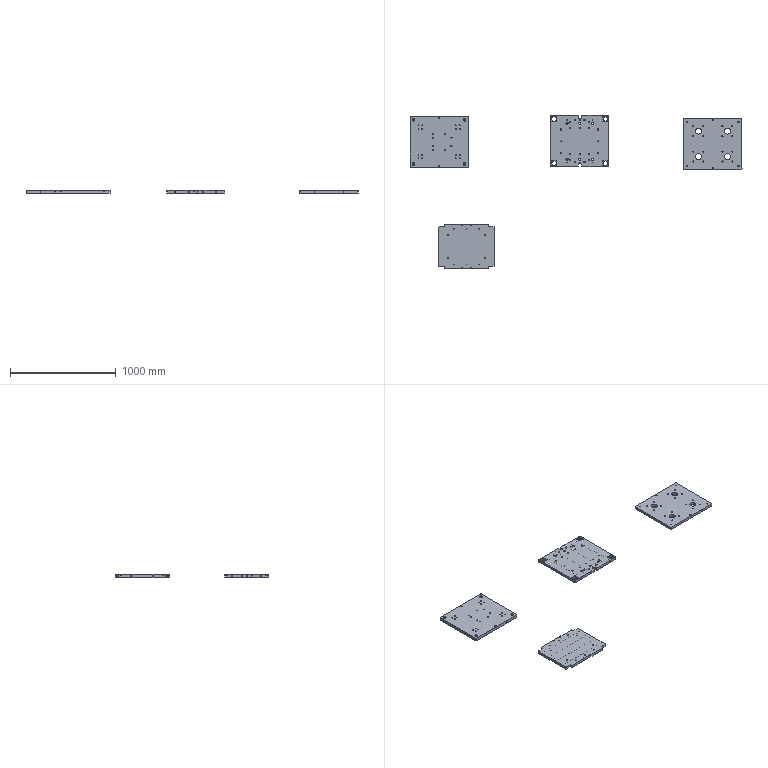NC program | Mastercam | posted with a generic post | part box 3140 x 1452 x 30 mm
Lines 481 to 2018 of 5015:
N4780 T16 M6
N4790 G0 G90 G17 G54 X-276. Y206. A0. S6000 M3
N4800 G43 H16 Z50. M8
N4810 Z1.
N4820 G1 Z-.499 F600.
N4830 X-260. F4000.
N4840 X-226.
N4850 Y212.5
N4860 Y228.5
N4870 Z-.998 F600.
N4880 Y212.5 F4000.
N4890 Y206.
N4900 X-260.
N4910 X-276.
N4920 Z-1.497 F600.
N4930 X-260. F4000.
N4940 X-226.
N4950 Y212.5
N4960 Y228.5
N4970 Z-1.996 F600.
N4980 Y212.5 F4000.
N4990 Y206.
N5000 X-260.
N5010 X-276.
N5020 Z-2.495 F600.
N5030 X-260. F4000.
N5040 X-226.
N5050 Y212.5
N5060 Y228.5
N5070 Z-2.994 F600.
N5080 Y212.5 F4000.
N5090 Y206.
N5100 X-260.
N5110 X-276.
N5120 Z-3.493 F600.
N5130 X-260. F4000.
N5140 X-226.
N5150 Y212.5
N5160 Y228.5
N5170 Z-3.992 F600.
N5180 Y212.5 F4000.
N5190 Y206.
N5200 X-260.
N5210 X-276.
N5220 Z-4.491 F600.
N5230 X-260. F4000.
N5240 X-226.
N5250 Y212.5
N5260 Y228.5
N5270 Z-4.99 F600.
N5280 Y212.5 F4000.
N5290 Y206.
N5300 X-260.
N5310 X-276.
N5320 Z-5.489 F600.
N5330 X-260. F4000.
N5340 X-226.
N5350 Y212.5
N5360 Y228.5
N5370 Z-5.988 F600.
N5380 Y212.5 F4000.
N5390 Y206.
N5400 X-260.
N5410 X-276.
N5420 Z-6.487 F600.
N5430 X-260. F4000.
N5440 X-226.
N5450 Y212.5
N5460 Y228.5
N5470 Z-6.986 F600.
N5480 Y212.5 F4000.
N5490 Y206.
N5500 X-260.
N5510 X-276.
N5520 Z-7.485 F600.
N5530 X-260. F4000.
N5540 X-226.
N5550 Y212.5
N5560 Y228.5
N5570 Z-7.984 F600.
N5580 Y212.5 F4000.
N5590 Y206.
N5600 X-260.
N5610 X-276.
N5620 Z-8.483 F600.
N5630 X-260. F4000.
N5640 X-226.
N5650 Y212.5
N5660 Y228.5
N5670 Z-8.982 F600.
N5680 Y212.5 F4000.
N5690 Y206.
N5700 X-260.
N5710 X-276.
N5720 Z-9.481 F600.
N5730 X-260. F4000.
N5740 X-226.
N5750 Y212.5
N5760 Y228.5
N5770 Z-9.98 F600.
N5780 Y212.5 F4000.
N5790 Y206.
N5800 X-260.
N5810 X-276.
N5820 Z-10.479 F600.
N5830 X-260. F4000.
N5840 X-226.
N5850 Y212.5
N5860 Y228.5
N5870 Z-10.978 F600.
N5880 Y212.5 F4000.
N5890 Y206.
N5900 X-260.
N5910 X-276.
N5920 Z-11.477 F600.
N5930 X-260. F4000.
N5940 X-226.
N5950 Y212.5
N5960 Y228.5
N5970 Z-11.976 F600.
N5980 Y212.5 F4000.
N5990 Y206.
N6000 X-260.
N6010 X-276.
N6020 Z-12.475 F600.
N6030 X-260. F4000.
N6040 X-226.
N6050 Y212.5
N6060 Y228.5
N6070 Z-12.974 F600.
N6080 Y212.5 F4000.
N6090 Y206.
N6100 X-260.
N6110 X-276.
N6120 Z-13.473 F600.
N6130 X-260. F4000.
N6140 X-226.
N6150 Y212.5
N6160 Y228.5
N6170 Z-13.972 F600.
N6180 Y212.5 F4000.
N6190 Y206.
N6200 X-260.
N6210 X-276.
N6220 Z-14.471 F600.
N6230 X-260. F4000.
N6240 X-226.
N6250 Y212.5
N6260 Y228.5
N6270 Z-14.97 F600.
N6280 Y212.5 F4000.
N6290 Y206.
N6300 X-260.
N6310 X-276.
N6320 Z-15.469 F600.
N6330 X-260. F4000.
N6340 X-226.
N6350 Y212.5
N6360 Y228.5
N6370 Z-15.968 F600.
N6380 Y212.5 F4000.
N6390 Y206.
N6400 X-260.
N6410 X-276.
N6420 Z-16.467 F600.
N6430 X-260. F4000.
N6440 X-226.
N6450 Y212.5
N6460 Y228.5
N6470 Z-16.966 F600.
N6480 Y212.5 F4000.
N6490 Y206.
N6500 X-260.
N6510 X-276.
N6520 Z-17.465 F600.
N6530 X-260. F4000.
N6540 X-226.
N6550 Y212.5
N6560 Y228.5
N6570 Z-17.964 F600.
N6580 Y212.5 F4000.
N6590 Y206.
N6600 X-260.
N6610 X-276.
N6620 Z-18.463 F600.
N6630 X-260. F4000.
N6640 X-226.
N6650 Y212.5
N6660 Y228.5
N6670 Z-18.962 F600.
N6680 Y212.5 F4000.
N6690 Y206.
N6700 X-260.
N6710 X-276.
N6720 Z-19.461 F600.
N6730 X-260. F4000.
N6740 X-226.
N6750 Y212.5
N6760 Y228.5
N6770 Z-19.96 F600.
N6780 Y212.5 F4000.
N6790 Y206.
N6800 X-260.
N6810 X-276.
N6820 Z-20.459 F600.
N6830 X-260. F4000.
N6840 X-226.
N6850 Y212.5
N6860 Y228.5
N6870 Z-20.958 F600.
N6880 Y212.5 F4000.
N6890 Y206.
N6900 X-260.
N6910 X-276.
N6920 Z-21.457 F600.
N6930 X-260. F4000.
N6940 X-226.
N6950 Y212.5
N6960 Y228.5
N6970 Z-21.956 F600.
N6980 Y212.5 F4000.
N6990 Y206.
N7000 X-260.
N7010 X-276.
N7020 Z-22.455 F600.
N7030 X-260. F4000.
N7040 X-226.
N7050 Y212.5
N7060 Y228.5
N7070 Z-22.954 F600.
N7080 Y212.5 F4000.
N7090 Y206.
N7100 X-260.
N7110 X-276.
N7120 Z-23.453 F600.
N7130 X-260. F4000.
N7140 X-226.
N7150 Y212.5
N7160 Y228.5
N7170 Z-23.952 F600.
N7180 Y212.5 F4000.
N7190 Y206.
N7200 X-260.
N7210 X-276.
N7220 Z-24.451 F600.
N7230 X-260. F4000.
N7240 X-226.
N7250 Y212.5
N7260 Y228.5
N7270 Z-24.95 F600.
N7280 Y212.5 F4000.
N7290 Y206.
N7300 X-260.
N7310 X-276.
N7320 G0 Z50.
N7330 Y198.
N7340 Z1.
N7350 G1 Z-.499 F600.
N7360 X-260. F4000.
N7370 X-218.
N7380 Y212.5
N7390 Y228.5
N7400 Z-.998 F600.
N7410 Y212.5 F4000.
N7420 Y198.
N7430 X-260.
N7440 X-276.
N7450 Z-1.497 F600.
N7460 X-260. F4000.
N7470 X-218.
N7480 Y212.5
N7490 Y228.5
N7500 Z-1.996 F600.
N7510 Y212.5 F4000.
N7520 Y198.
N7530 X-260.
N7540 X-276.
N7550 Z-2.495 F600.
N7560 X-260. F4000.
N7570 X-218.
N7580 Y212.5
N7590 Y228.5
N7600 Z-2.994 F600.
N7610 Y212.5 F4000.
N7620 Y198.
N7630 X-260.
N7640 X-276.
N7650 Z-3.493 F600.
N7660 X-260. F4000.
N7670 X-218.
N7680 Y212.5
N7690 Y228.5
N7700 Z-3.992 F600.
N7710 Y212.5 F4000.
N7720 Y198.
N7730 X-260.
N7740 X-276.
N7750 Z-4.491 F600.
N7760 X-260. F4000.
N7770 X-218.
N7780 Y212.5
N7790 Y228.5
N7800 Z-4.99 F600.
N7810 Y212.5 F4000.
N7820 Y198.
N7830 X-260.
N7840 X-276.
N7850 Z-5.489 F600.
N7860 X-260. F4000.
N7870 X-218.
N7880 Y212.5
N7890 Y228.5
N7900 Z-5.988 F600.
N7910 Y212.5 F4000.
N7920 Y198.
N7930 X-260.
N7940 X-276.
N7950 Z-6.487 F600.
N7960 X-260. F4000.
N7970 X-218.
N7980 Y212.5
N7990 Y228.5
N8000 Z-6.986 F600.
N8010 Y212.5 F4000.
N8020 Y198.
N8030 X-260.
N8040 X-276.
N8050 Z-7.485 F600.
N8060 X-260. F4000.
N8070 X-218.
N8080 Y212.5
N8090 Y228.5
N8100 Z-7.984 F600.
N8110 Y212.5 F4000.
N8120 Y198.
N8130 X-260.
N8140 X-276.
N8150 Z-8.483 F600.
N8160 X-260. F4000.
N8170 X-218.
N8180 Y212.5
N8190 Y228.5
N8200 Z-8.982 F600.
N8210 Y212.5 F4000.
N8220 Y198.
N8230 X-260.
N8240 X-276.
N8250 Z-9.481 F600.
N8260 X-260. F4000.
N8270 X-218.
N8280 Y212.5
N8290 Y228.5
N8300 Z-9.98 F600.
N8310 Y212.5 F4000.
N8320 Y198.
N8330 X-260.
N8340 X-276.
N8350 Z-10.479 F600.
N8360 X-260. F4000.
N8370 X-218.
N8380 Y212.5
N8390 Y228.5
N8400 Z-10.978 F600.
N8410 Y212.5 F4000.
N8420 Y198.
N8430 X-260.
N8440 X-276.
N8450 Z-11.477 F600.
N8460 X-260. F4000.
N8470 X-218.
N8480 Y212.5
N8490 Y228.5
N8500 Z-11.976 F600.
N8510 Y212.5 F4000.
N8520 Y198.
N8530 X-260.
N8540 X-276.
N8550 Z-12.475 F600.
N8560 X-260. F4000.
N8570 X-218.
N8580 Y212.5
N8590 Y228.5
N8600 Z-12.974 F600.
N8610 Y212.5 F4000.
N8620 Y198.
N8630 X-260.
N8640 X-276.
N8650 Z-13.473 F600.
N8660 X-260. F4000.
N8670 X-218.
N8680 Y212.5
N8690 Y228.5
N8700 Z-13.972 F600.
N8710 Y212.5 F4000.
N8720 Y198.
N8730 X-260.
N8740 X-276.
N8750 Z-14.471 F600.
N8760 X-260. F4000.
N8770 X-218.
N8780 Y212.5
N8790 Y228.5
N8800 Z-14.97 F600.
N8810 Y212.5 F4000.
N8820 Y198.
N8830 X-260.
N8840 X-276.
N8850 Z-15.469 F600.
N8860 X-260. F4000.
N8870 X-218.
N8880 Y212.5
N8890 Y228.5
N8900 Z-15.968 F600.
N8910 Y212.5 F4000.
N8920 Y198.
N8930 X-260.
N8940 X-276.
N8950 Z-16.467 F600.
N8960 X-260. F4000.
N8970 X-218.
N8980 Y212.5
N8990 Y228.5
N9000 Z-16.966 F600.
N9010 Y212.5 F4000.
N9020 Y198.
N9030 X-260.
N9040 X-276.
N9050 Z-17.465 F600.
N9060 X-260. F4000.
N9070 X-218.
N9080 Y212.5
N9090 Y228.5
N9100 Z-17.964 F600.
N9110 Y212.5 F4000.
N9120 Y198.
N9130 X-260.
N9140 X-276.
N9150 Z-18.463 F600.
N9160 X-260. F4000.
N9170 X-218.
N9180 Y212.5
N9190 Y228.5
N9200 Z-18.962 F600.
N9210 Y212.5 F4000.
N9220 Y198.
N9230 X-260.
N9240 X-276.
N9250 Z-19.461 F600.
N9260 X-260. F4000.
N9270 X-218.
N9280 Y212.5
N9290 Y228.5
N9300 Z-19.96 F600.
N9310 Y212.5 F4000.
N9320 Y198.
N9330 X-260.
N9340 X-276.
N9350 Z-20.459 F600.
N9360 X-260. F4000.
N9370 X-218.
N9380 Y212.5
N9390 Y228.5
N9400 Z-20.958 F600.
N9410 Y212.5 F4000.
N9420 Y198.
N9430 X-260.
N9440 X-276.
N9450 Z-21.457 F600.
N9460 X-260. F4000.
N9470 X-218.
N9480 Y212.5
N9490 Y228.5
N9500 Z-21.956 F600.
N9510 Y212.5 F4000.
N9520 Y198.
N9530 X-260.
N9540 X-276.
N9550 Z-22.455 F600.
N9560 X-260. F4000.
N9570 X-218.
N9580 Y212.5
N9590 Y228.5
N9600 Z-22.954 F600.
N9610 Y212.5 F4000.
N9620 Y198.
N9630 X-260.
N9640 X-276.
N9650 Z-23.453 F600.
N9660 X-260. F4000.
N9670 X-218.
N9680 Y212.5
N9690 Y228.5
N9700 Z-23.952 F600.
N9710 Y212.5 F4000.
N9720 Y198.
N9730 X-260.
N9740 X-276.
N9750 Z-24.451 F600.
N9760 X-260. F4000.
N9770 X-218.
N9780 Y212.5
N9790 Y228.5
N9800 Z-24.95 F600.
N9810 Y212.5 F4000.
N9820 Y198.
N9830 X-260.
N9840 X-276.
N9850 G0 Z50.
N9860 X226. Y228.5
N9870 Z1.
N9880 G1 Z-.499 F600.
N9890 Y212.5 F4000.
N9900 Y206.
N9910 X260.
N9920 X276.
N9930 Z-.998 F600.
N9940 X260. F4000.
N9950 X226.
N9960 Y212.5
N9970 Y228.5
N9980 Z-1.497 F600.
N9990 Y212.5 F4000.
N100 Y206.
N110 X260.
N120 X276.
N130 Z-1.996 F600.
N140 X260. F4000.
N150 X226.
N160 Y212.5
N170 Y228.5
N180 Z-2.495 F600.
N190 Y212.5 F4000.
N200 Y206.
N210 X260.
N220 X276.
N230 Z-2.994 F600.
N240 X260. F4000.
N250 X226.
N260 Y212.5
N270 Y228.5
N280 Z-3.493 F600.
N290 Y212.5 F4000.
N300 Y206.
N310 X260.
N320 X276.
N330 Z-3.992 F600.
N340 X260. F4000.
N350 X226.
N360 Y212.5
N370 Y228.5
N380 Z-4.491 F600.
N390 Y212.5 F4000.
N400 Y206.
N410 X260.
N420 X276.
N430 Z-4.99 F600.
N440 X260. F4000.
N450 X226.
N460 Y212.5
N470 Y228.5
N480 Z-5.489 F600.
N490 Y212.5 F4000.
N500 Y206.
N510 X260.
N520 X276.
N530 Z-5.988 F600.
N540 X260. F4000.
N550 X226.
N560 Y212.5
N570 Y228.5
N580 Z-6.487 F600.
N590 Y212.5 F4000.
N600 Y206.
N610 X260.
N620 X276.
N630 Z-6.986 F600.
N640 X260. F4000.
N650 X226.
N660 Y212.5
N670 Y228.5
N680 Z-7.485 F600.
N690 Y212.5 F4000.
N700 Y206.
N710 X260.
N720 X276.
N730 Z-7.984 F600.
N740 X260. F4000.
N750 X226.
N760 Y212.5
N770 Y228.5
N780 Z-8.483 F600.
N790 Y212.5 F4000.
N800 Y206.
N810 X260.
N820 X276.
N830 Z-8.982 F600.
N840 X260. F4000.
N850 X226.
N860 Y212.5
N870 Y228.5
N880 Z-9.481 F600.
N890 Y212.5 F4000.
N900 Y206.
N910 X260.
N920 X276.
N930 Z-9.98 F600.
N940 X260. F4000.
N950 X226.
N960 Y212.5
N970 Y228.5
N980 Z-10.479 F600.
N990 Y212.5 F4000.
N1000 Y206.
N1010 X260.
N1020 X276.
N1030 Z-10.978 F600.
N1040 X260. F4000.
N1050 X226.
N1060 Y212.5
N1070 Y228.5
N1080 Z-11.477 F600.
N1090 Y212.5 F4000.
N1100 Y206.
N1110 X260.
N1120 X276.
N1130 Z-11.976 F600.
N1140 X260. F4000.
N1150 X226.
N1160 Y212.5
N1170 Y228.5
N1180 Z-12.475 F600.
N1190 Y212.5 F4000.
N1200 Y206.
N1210 X260.
N1220 X276.
N1230 Z-12.974 F600.
N1240 X260. F4000.
N1250 X226.
N1260 Y212.5
N1270 Y228.5
N1280 Z-13.473 F600.
N1290 Y212.5 F4000.
N1300 Y206.
N1310 X260.
N1320 X276.
N1330 Z-13.972 F600.
N1340 X260. F4000.
N1350 X226.
N1360 Y212.5
N1370 Y228.5
N1380 Z-14.471 F600.
N1390 Y212.5 F4000.
N1400 Y206.
N1410 X260.
N1420 X276.
N1430 Z-14.97 F600.
N1440 X260. F4000.
N1450 X226.
N1460 Y212.5
N1470 Y228.5
N1480 Z-15.469 F600.
N1490 Y212.5 F4000.
N1500 Y206.
N1510 X260.
N1520 X276.
N1530 Z-15.968 F600.
N1540 X260. F4000.
N1550 X226.
N1560 Y212.5
N1570 Y228.5
N1580 Z-16.467 F600.
N1590 Y212.5 F4000.
N1600 Y206.
N1610 X260.
N1620 X276.
N1630 Z-16.966 F600.
N1640 X260. F4000.
N1650 X226.
N1660 Y212.5
N1670 Y228.5
N1680 Z-17.465 F600.
N1690 Y212.5 F4000.
N1700 Y206.
N1710 X260.
N1720 X276.
N1730 Z-17.964 F600.
N1740 X260. F4000.
N1750 X226.
N1760 Y212.5
N1770 Y228.5
N1780 Z-18.463 F600.
N1790 Y212.5 F4000.
N1800 Y206.
N1810 X260.
N1820 X276.
N1830 Z-18.962 F600.
N1840 X260. F4000.
N1850 X226.
N1860 Y212.5
N1870 Y228.5
N1880 Z-19.461 F600.
N1890 Y212.5 F4000.
N1900 Y206.
N1910 X260.
N1920 X276.
N1930 Z-19.96 F600.
N1940 X260. F4000.
N1950 X226.
N1960 Y212.5
N1970 Y228.5
N1980 Z-20.459 F600.
N1990 Y212.5 F4000.
N2000 Y206.
N2010 X260.
N2020 X276.
N2030 Z-20.958 F600.
N2040 X260. F4000.
N2050 X226.
N2060 Y212.5
N2070 Y228.5
N2080 Z-21.457 F600.
N2090 Y212.5 F4000.
N2100 Y206.
N2110 X260.
N2120 X276.
N2130 Z-21.956 F600.
N2140 X260. F4000.
N2150 X226.
N2160 Y212.5
N2170 Y228.5
N2180 Z-22.455 F600.
N2190 Y212.5 F4000.
N2200 Y206.
N2210 X260.
N2220 X276.
N2230 Z-22.954 F600.
N2240 X260. F4000.
N2250 X226.
N2260 Y212.5
N2270 Y228.5
N2280 Z-23.453 F600.
N2290 Y212.5 F4000.
N2300 Y206.
N2310 X260.
N2320 X276.
N2330 Z-23.952 F600.
N2340 X260. F4000.
N2350 X226.
N2360 Y212.5
N2370 Y228.5
N2380 Z-24.451 F600.
N2390 Y212.5 F4000.
N2400 Y206.
N2410 X260.
N2420 X276.
N2430 Z-24.95 F600.
N2440 X260. F4000.
N2450 X226.
N2460 Y212.5
N2470 Y228.5
N2480 G0 Z50.
N2490 X218.
N2500 Z1.
N2510 G1 Z-.499 F600.
N2520 Y212.5 F4000.
N2530 Y198.
N2540 X260.
N2550 X276.
N2560 Z-.998 F600.
N2570 X260. F4000.
N2580 X218.
N2590 Y212.5
N2600 Y228.5
N2610 Z-1.497 F600.
N2620 Y212.5 F4000.
N2630 Y198.
N2640 X260.
N2650 X276.
N2660 Z-1.996 F600.
N2670 X260. F4000.
N2680 X218.
N2690 Y212.5
N2700 Y228.5
N2710 Z-2.495 F600.
N2720 Y212.5 F4000.
N2730 Y198.
N2740 X260.
N2750 X276.
N2760 Z-2.994 F600.
N2770 X260. F4000.
N2780 X218.
N2790 Y212.5
N2800 Y228.5
N2810 Z-3.493 F600.
N2820 Y212.5 F4000.
N2830 Y198.
N2840 X260.
N2850 X276.
N2860 Z-3.992 F600.
N2870 X260. F4000.
N2880 X218.
N2890 Y212.5
N2900 Y228.5
N2910 Z-4.491 F600.
N2920 Y212.5 F4000.
N2930 Y198.
N2940 X260.
N2950 X276.
N2960 Z-4.99 F600.
N2970 X260. F4000.
N2980 X218.
N2990 Y212.5
N3000 Y228.5
N3010 Z-5.489 F600.
N3020 Y212.5 F4000.
N3030 Y198.
N3040 X260.
N3050 X276.
N3060 Z-5.988 F600.
N3070 X260. F4000.
N3080 X218.
N3090 Y212.5
N3100 Y228.5
N3110 Z-6.487 F600.
N3120 Y212.5 F4000.
N3130 Y198.
N3140 X260.
N3150 X276.
N3160 Z-6.986 F600.
N3170 X260. F4000.
N3180 X218.
N3190 Y212.5
N3200 Y228.5
N3210 Z-7.485 F600.
N3220 Y212.5 F4000.
N3230 Y198.
N3240 X260.
N3250 X276.
N3260 Z-7.984 F600.
N3270 X260. F4000.
N3280 X218.
N3290 Y212.5
N3300 Y228.5
N3310 Z-8.483 F600.
N3320 Y212.5 F4000.
N3330 Y198.
N3340 X260.
N3350 X276.
N3360 Z-8.982 F600.
N3370 X260. F4000.
N3380 X218.
N3390 Y212.5
N3400 Y228.5
N3410 Z-9.481 F600.
N3420 Y212.5 F4000.
N3430 Y198.
N3440 X260.
N3450 X276.
N3460 Z-9.98 F600.
N3470 X260. F4000.
N3480 X218.
N3490 Y212.5
N3500 Y228.5
N3510 Z-10.479 F600.
N3520 Y212.5 F4000.
N3530 Y198.
N3540 X260.
N3550 X276.
N3560 Z-10.978 F600.
N3570 X260. F4000.
N3580 X218.
N3590 Y212.5
N3600 Y228.5
N3610 Z-11.477 F600.
N3620 Y212.5 F4000.
N3630 Y198.
N3640 X260.
N3650 X276.
N3660 Z-11.976 F600.
N3670 X260. F4000.
N3680 X218.
N3690 Y212.5
N3700 Y228.5
N3710 Z-12.475 F600.
N3720 Y212.5 F4000.
N3730 Y198.
N3740 X260.
N3750 X276.
N3760 Z-12.974 F600.
N3770 X260. F4000.
N3780 X218.
N3790 Y212.5
N3800 Y228.5
N3810 Z-13.473 F600.
N3820 Y212.5 F4000.
N3830 Y198.
N3840 X260.
N3850 X276.
N3860 Z-13.972 F600.
N3870 X260. F4000.
N3880 X218.
N3890 Y212.5
N3900 Y228.5
N3910 Z-14.471 F600.
N3920 Y212.5 F4000.
N3930 Y198.
N3940 X260.
N3950 X276.
N3960 Z-14.97 F600.
N3970 X260. F4000.
N3980 X218.
N3990 Y212.5
N4000 Y228.5
N4010 Z-15.469 F600.
N4020 Y212.5 F4000.
N4030 Y198.
N4040 X260.
N4050 X276.
N4060 Z-15.968 F600.
N4070 X260. F4000.
N4080 X218.
N4090 Y212.5
N4100 Y228.5
N4110 Z-16.467 F600.
N4120 Y212.5 F4000.
N4130 Y198.
N4140 X260.
N4150 X276.
N4160 Z-16.966 F600.
N4170 X260. F4000.
N4180 X218.
N4190 Y212.5
N4200 Y228.5
N4210 Z-17.465 F600.
N4220 Y212.5 F4000.
N4230 Y198.
N4240 X260.
N4250 X276.
N4260 Z-17.964 F600.
N4270 X260. F4000.
N4280 X218.
N4290 Y212.5
N4300 Y228.5
N4310 Z-18.463 F600.
N4320 Y212.5 F4000.
N4330 Y198.
N4340 X260.
N4350 X276.
N4360 Z-18.962 F600.
N4370 X260. F4000.
N4380 X218.
N4390 Y212.5
N4400 Y228.5
N4410 Z-19.461 F600.
N4420 Y212.5 F4000.
N4430 Y198.
N4440 X260.
N4450 X276.
N4460 Z-19.96 F600.
N4470 X260. F4000.
N4480 X218.
N4490 Y212.5
N4500 Y228.5
N4510 Z-20.459 F600.
N4520 Y212.5 F4000.
N4530 Y198.
N4540 X260.
N4550 X276.
N4560 Z-20.958 F600.
N4570 X260. F4000.
N4580 X218.
N4590 Y212.5
N4600 Y228.5
N4610 Z-21.457 F600.
N4620 Y212.5 F4000.
N4630 Y198.
N4640 X260.
N4650 X276.
N4660 Z-21.956 F600.
N4670 X260. F4000.
N4680 X218.
N4690 Y212.5
N4700 Y228.5
N4710 Z-22.455 F600.
N4720 Y212.5 F4000.
N4730 Y198.
N4740 X260.
N4750 X276.
N4760 Z-22.954 F600.
N4770 X260. F4000.
N4780 X218.
N4790 Y212.5
N4800 Y228.5
N4810 Z-23.453 F600.
N4820 Y212.5 F4000.
N4830 Y198.
N4840 X260.
N4850 X276.
N4860 Z-23.952 F600.
N4870 X260. F4000.
N4880 X218.
N4890 Y212.5
N4900 Y228.5
N4910 Z-24.451 F600.
N4920 Y212.5 F4000.
N4930 Y198.
N4940 X260.
N4950 X276.
N4960 Z-24.95 F600.
N4970 X260. F4000.
N4980 X218.
N4990 Y212.5
N5000 Y228.5
N5010 G0 Z50.
N5020 X276. Y-206.
N5030 Z1.
N5040 G1 Z-.499 F600.
N5050 X260. F4000.
N5060 X226.
N5070 Y-212.5
N5080 Y-228.5
N5090 Z-.998 F600.
N5100 Y-212.5 F4000.
N5110 Y-206.
N5120 X260.
N5130 X276.
N5140 Z-1.497 F600.
N5150 X260. F4000.
N5160 X226.
N5170 Y-212.5
N5180 Y-228.5
N5190 Z-1.996 F600.
N5200 Y-212.5 F4000.
N5210 Y-206.
N5220 X260.
N5230 X276.
N5240 Z-2.495 F600.
N5250 X260. F4000.
N5260 X226.
N5270 Y-212.5
N5280 Y-228.5
N5290 Z-2.994 F600.
N5300 Y-212.5 F4000.
N5310 Y-206.
N5320 X260.
N5330 X276.
N5340 Z-3.493 F600.
N5350 X260. F4000.
N5360 X226.
N5370 Y-212.5
N5380 Y-228.5
N5390 Z-3.992 F600.
N5400 Y-212.5 F4000.
N5410 Y-206.
N5420 X260.
N5430 X276.
N5440 Z-4.491 F600.
N5450 X260. F4000.
N5460 X226.
N5470 Y-212.5
N5480 Y-228.5
N5490 Z-4.99 F600.
N5500 Y-212.5 F4000.
N5510 Y-206.
N5520 X260.
N5530 X276.
N5540 Z-5.489 F600.
N5550 X260. F4000.
N5560 X226.
N5570 Y-212.5
N5580 Y-228.5
N5590 Z-5.988 F600.
N5600 Y-212.5 F4000.
N5610 Y-206.
N5620 X260.
N5630 X276.
N5640 Z-6.487 F600.
N5650 X260. F4000.
N5660 X226.
N5670 Y-212.5
N5680 Y-228.5
N5690 Z-6.986 F600.
N5700 Y-212.5 F4000.
N5710 Y-206.
N5720 X260.
N5730 X276.
N5740 Z-7.485 F600.
N5750 X260. F4000.
N5760 X226.
N5770 Y-212.5
N5780 Y-228.5
N5790 Z-7.984 F600.
N5800 Y-212.5 F4000.
N5810 Y-206.
N5820 X260.
N5830 X276.
N5840 Z-8.483 F600.
N5850 X260. F4000.
N5860 X226.
N5870 Y-212.5
N5880 Y-228.5
N5890 Z-8.982 F600.
N5900 Y-212.5 F4000.
N5910 Y-206.
N5920 X260.
N5930 X276.
N5940 Z-9.481 F600.
N5950 X260. F4000.
N5960 X226.
N5970 Y-212.5
N5980 Y-228.5
N5990 Z-9.98 F600.
N6000 Y-212.5 F4000.
N6010 Y-206.
N6020 X260.
N6030 X276.
N6040 Z-10.479 F600.
N6050 X260. F4000.
N6060 X226.
N6070 Y-212.5
N6080 Y-228.5
N6090 Z-10.978 F600.
N6100 Y-212.5 F4000.
N6110 Y-206.
N6120 X260.
N6130 X276.
N6140 Z-11.477 F600.
N6150 X260. F4000.
N6160 X226.
N6170 Y-212.5
N6180 Y-228.5
N6190 Z-11.976 F600.
N6200 Y-212.5 F4000.
N6210 Y-206.
N6220 X260.
N6230 X276.
N6240 Z-12.475 F600.
N6250 X260. F4000.
N6260 X226.
N6270 Y-212.5
N6280 Y-228.5
N6290 Z-12.974 F600.
N6300 Y-212.5 F4000.
N6310 Y-206.
N6320 X260.
N6330 X276.
N6340 Z-13.473 F600.
N6350 X260. F4000.
N6360 X226.
N6370 Y-212.5
N6380 Y-228.5
N6390 Z-13.972 F600.
N6400 Y-212.5 F4000.
N6410 Y-206.
N6420 X260.
N6430 X276.
N6440 Z-14.471 F600.
N6450 X260. F4000.
N6460 X226.
N6470 Y-212.5
N6480 Y-228.5
N6490 Z-14.97 F600.
N6500 Y-212.5 F4000.
N6510 Y-206.
N6520 X260.
N6530 X276.
N6540 Z-15.469 F600.
N6550 X260. F4000.
N6560 X226.
N6570 Y-212.5
N6580 Y-228.5
N6590 Z-15.968 F600.
N6600 Y-212.5 F4000.
N6610 Y-206.
N6620 X260.
N6630 X276.
N6640 Z-16.467 F600.
N6650 X260. F4000.
N6660 X226.
N6670 Y-212.5
N6680 Y-228.5
N6690 Z-16.966 F600.
N6700 Y-212.5 F4000.
N6710 Y-206.
N6720 X260.
N6730 X276.
N6740 Z-17.465 F600.
N6750 X260. F4000.
N6760 X226.
N6770 Y-212.5
N6780 Y-228.5
N6790 Z-17.964 F600.
N6800 Y-212.5 F4000.
N6810 Y-206.
N6820 X260.
N6830 X276.
N6840 Z-18.463 F600.
N6850 X260. F4000.
N6860 X226.
N6870 Y-212.5
N6880 Y-228.5
N6890 Z-18.962 F600.
N6900 Y-212.5 F4000.
N6910 Y-206.
N6920 X260.
N6930 X276.
N6940 Z-19.461 F600.
N6950 X260. F4000.
N6960 X226.
N6970 Y-212.5
N6980 Y-228.5
N6990 Z-19.96 F600.
N7000 Y-212.5 F4000.
N7010 Y-206.
N7020 X260.
N7030 X276.
N7040 Z-20.459 F600.
N7050 X260. F4000.
N7060 X226.
N7070 Y-212.5
N7080 Y-228.5
N7090 Z-20.958 F600.
N7100 Y-212.5 F4000.
N7110 Y-206.
N7120 X260.
N7130 X276.
N7140 Z-21.457 F600.
N7150 X260. F4000.
N7160 X226.
N7170 Y-212.5
N7180 Y-228.5
N7190 Z-21.956 F600.
N7200 Y-212.5 F4000.
N7210 Y-206.
N7220 X260.
N7230 X276.
N7240 Z-22.455 F600.
N7250 X260. F4000.
N7260 X226.
N7270 Y-212.5
N7280 Y-228.5
N7290 Z-22.954 F600.
N7300 Y-212.5 F4000.
N7310 Y-206.
N7320 X260.
N7330 X276.
N7340 Z-23.453 F600.
N7350 X260. F4000.
N7360 X226.
N7370 Y-212.5
N7380 Y-228.5
N7390 Z-23.952 F600.
N7400 Y-212.5 F4000.
N7410 Y-206.
N7420 X260.
N7430 X276.
N7440 Z-24.451 F600.
N7450 X260. F4000.
N7460 X226.
N7470 Y-212.5
N7480 Y-228.5
N7490 Z-24.95 F600.
N7500 Y-212.5 F4000.
N7510 Y-206.
N7520 X260.
N7530 X276.
N7540 G0 Z50.
N7550 Y-198.
N7560 Z1.
N7570 G1 Z-.499 F600.
N7580 X260. F4000.
N7590 X218.
N7600 Y-212.5
N7610 Y-228.5
N7620 Z-.998 F600.
N7630 Y-212.5 F4000.
N7640 Y-198.
N7650 X260.
N7660 X276.
N7670 Z-1.497 F600.
N7680 X260. F4000.
N7690 X218.
N7700 Y-212.5
N7710 Y-228.5
N7720 Z-1.996 F600.
N7730 Y-212.5 F4000.
N7740 Y-198.
N7750 X260.
N7760 X276.
N7770 Z-2.495 F600.
N7780 X260. F4000.
N7790 X218.
N7800 Y-212.5
N7810 Y-228.5
N7820 Z-2.994 F600.
N7830 Y-212.5 F4000.
N7840 Y-198.
N7850 X260.
N7860 X276.
N7870 Z-3.493 F600.
N7880 X260. F4000.
N7890 X218.
N7900 Y-212.5
N7910 Y-228.5
N7920 Z-3.992 F600.
N7930 Y-212.5 F4000.
N7940 Y-198.
N7950 X260.
N7960 X276.
N7970 Z-4.491 F600.
N7980 X260. F4000.
N7990 X218.
N8000 Y-212.5
N8010 Y-228.5
N8020 Z-4.99 F600.
N8030 Y-212.5 F4000.
N8040 Y-198.
N8050 X260.
N8060 X276.
N8070 Z-5.489 F600.
N8080 X260. F4000.
N8090 X218.
N8100 Y-212.5
N8110 Y-228.5
N8120 Z-5.988 F600.
N8130 Y-212.5 F4000.
N8140 Y-198.
N8150 X260.
N8160 X276.
N8170 Z-6.487 F600.
N8180 X260. F4000.
N8190 X218.
N8200 Y-212.5
N8210 Y-228.5
N8220 Z-6.986 F600.
N8230 Y-212.5 F4000.
N8240 Y-198.
N8250 X260.
N8260 X276.
N8270 Z-7.485 F600.
N8280 X260. F4000.
N8290 X218.
N8300 Y-212.5
N8310 Y-228.5
N8320 Z-7.984 F600.
N8330 Y-212.5 F4000.
N8340 Y-198.
N8350 X260.
N8360 X276.
N8370 Z-8.483 F600.
N8380 X260. F4000.
N8390 X218.
N8400 Y-212.5
N8410 Y-228.5
N8420 Z-8.982 F600.
N8430 Y-212.5 F4000.
N8440 Y-198.
N8450 X260.
N8460 X276.
N8470 Z-9.481 F600.
N8480 X260. F4000.
N8490 X218.
N8500 Y-212.5
N8510 Y-228.5
N8520 Z-9.98 F600.
N8530 Y-212.5 F4000.
N8540 Y-198.
N8550 X260.
N8560 X276.
N8570 Z-10.479 F600.
N8580 X260. F4000.
N8590 X218.
N8600 Y-212.5
N8610 Y-228.5
N8620 Z-10.978 F600.
N8630 Y-212.5 F4000.
N8640 Y-198.
N8650 X260.
N8660 X276.
N8670 Z-11.477 F600.
N8680 X260. F4000.
N8690 X218.
N8700 Y-212.5
N8710 Y-228.5
N8720 Z-11.976 F600.
N8730 Y-212.5 F4000.
N8740 Y-198.
N8750 X260.
N8760 X276.
N8770 Z-12.475 F600.
N8780 X260. F4000.
N8790 X218.
N8800 Y-212.5
N8810 Y-228.5
N8820 Z-12.974 F600.
N8830 Y-212.5 F4000.
N8840 Y-198.
N8850 X260.
N8860 X276.
N8870 Z-13.473 F600.
N8880 X260. F4000.
N8890 X218.
N8900 Y-212.5
N8910 Y-228.5
N8920 Z-13.972 F600.
N8930 Y-212.5 F4000.
N8940 Y-198.
N8950 X260.
N8960 X276.
N8970 Z-14.471 F600.
N8980 X260. F4000.
N8990 X218.
N9000 Y-212.5
N9010 Y-228.5
N9020 Z-14.97 F600.
N9030 Y-212.5 F4000.
N9040 Y-198.
N9050 X260.
N9060 X276.
N9070 Z-15.469 F600.
N9080 X260. F4000.
N9090 X218.
N9100 Y-212.5
N9110 Y-228.5
N9120 Z-15.968 F600.
N9130 Y-212.5 F4000.
N9140 Y-198.
N9150 X260.
N9160 X276.
N9170 Z-16.467 F600.
N9180 X260. F4000.
N9190 X218.
N9200 Y-212.5
N9210 Y-228.5
N9220 Z-16.966 F600.
N9230 Y-212.5 F4000.
N9240 Y-198.
N9250 X260.
N9260 X276.
N9270 Z-17.465 F600.
N9280 X260. F4000.
N9290 X218.
N9300 Y-212.5
N9310 Y-228.5
N9320 Z-17.964 F600.
N9330 Y-212.5 F4000.
N9340 Y-198.
N9350 X260.
N9360 X276.
N9370 Z-18.463 F600.
N9380 X260. F4000.
N9390 X218.
N9400 Y-212.5
N9410 Y-228.5
N9420 Z-18.962 F600.
N9430 Y-212.5 F4000.
N9440 Y-198.
N9450 X260.
N9460 X276.
N9470 Z-19.461 F600.
N9480 X260. F4000.
N9490 X218.
N9500 Y-212.5
N9510 Y-228.5
N9520 Z-19.96 F600.
N9530 Y-212.5 F4000.
N9540 Y-198.
N9550 X260.
N9560 X276.
N9570 Z-20.459 F600.
N9580 X260. F4000.
N9590 X218.
N9600 Y-212.5
N9610 Y-228.5
N9620 Z-20.958 F600.
N9630 Y-212.5 F4000.
N9640 Y-198.
N9650 X260.
N9660 X276.
N9670 Z-21.457 F600.
N9680 X260. F4000.
N9690 X218.
N9700 Y-212.5
N9710 Y-228.5
N9720 Z-21.956 F600.
N9730 Y-212.5 F4000.
N9740 Y-198.
N9750 X260.
N9760 X276.
N9770 Z-22.455 F600.
N9780 X260. F4000.
N9790 X218.
N9800 Y-212.5
N9810 Y-228.5
N9820 Z-22.954 F600.
N9830 Y-212.5 F4000.
N9840 Y-198.
N9850 X260.
N9860 X276.
N9870 Z-23.453 F600.
N9880 X260. F4000.
N9890 X218.
N9900 Y-212.5
N9910 Y-228.5
N9920 Z-23.952 F600.
N9930 Y-212.5 F4000.
N9940 Y-198.
N9950 X260.
N9960 X276.
N9970 Z-24.451 F600.
N9980 X260. F4000.
N9990 X218.
N100 Y-212.5
N110 Y-228.5
N120 Z-24.95 F600.
N130 Y-212.5 F4000.
N140 Y-198.
N150 X260.
N160 X276.
N170 G0 Z50.
N180 X-226. Y-228.5
N190 Z1.
N200 G1 Z-.499 F600.
N210 Y-212.5 F4000.
N220 Y-206.
N230 X-260.
N240 X-276.
N250 Z-.998 F600.
N260 X-260. F4000.
N270 X-226.
N280 Y-212.5
N290 Y-228.5
N300 Z-1.497 F600.
N310 Y-212.5 F4000.
N320 Y-206.
N330 X-260.
N340 X-276.
N350 Z-1.996 F600.